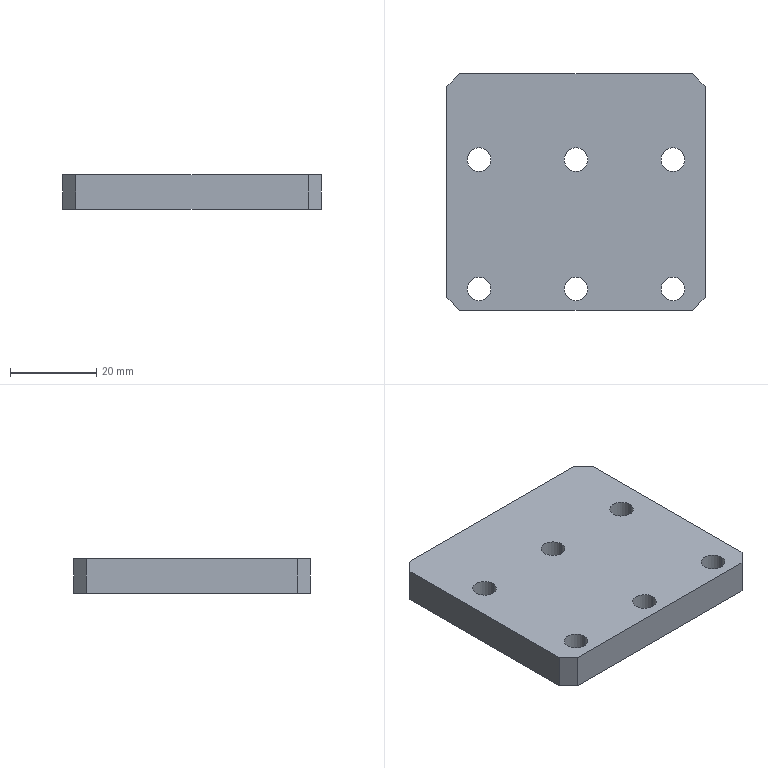Part | SolidWorks | features Chamfer 1, Extrusion 1, HoleWzd 1 | 1 solid | 22 faces | box 60 x 55 x 8 mm | volume 25116 mm3 | cylinder 12 | plane 10 | commonest cylinder face diameters 5.5 x12
STEP:
#1=CARTESIAN_POINT('',(-25.25,-22.5,0.));
#2=VERTEX_POINT('',#1);
#3=CARTESIAN_POINT('',(-19.75,-22.5,0.));
#4=VERTEX_POINT('',#3);
#5=CARTESIAN_POINT('',(-22.5,-22.5,0.));
#6=DIRECTION('',(0.,0.,1.));
#7=DIRECTION('',(1.,0.,0.));
#8=AXIS2_PLACEMENT_3D('',#5,#6,#7);
#9=CIRCLE('',#8,2.75);
#10=EDGE_CURVE('',#2,#4,#9,.T.);
#11=ORIENTED_EDGE('',*,*,#10,.F.);
#12=CARTESIAN_POINT('',(-25.25,-22.5,8.));
#13=VERTEX_POINT('',#12);
#14=CARTESIAN_POINT('',(-25.25,-22.5,8.));
#15=DIRECTION('',(0.,0.,1.));
#16=VECTOR('',#15,1000.);
#17=LINE('',#14,#16);
#18=EDGE_CURVE('',#2,#13,#17,.T.);
#19=ORIENTED_EDGE('',*,*,#18,.T.);
#20=CARTESIAN_POINT('',(-19.75,-22.5,8.));
#21=VERTEX_POINT('',#20);
#22=CARTESIAN_POINT('',(-22.5,-22.5,8.));
#23=DIRECTION('',(0.,0.,1.));
#24=DIRECTION('',(1.,0.,0.));
#25=AXIS2_PLACEMENT_3D('',#22,#23,#24);
#26=CIRCLE('',#25,2.75);
#27=EDGE_CURVE('',#13,#21,#26,.T.);
#28=ORIENTED_EDGE('',*,*,#27,.T.);
#29=CARTESIAN_POINT('',(-19.75,-22.5,8.));
#30=DIRECTION('',(0.,0.,1.));
#31=VECTOR('',#30,1000.);
#32=LINE('',#29,#31);
#33=EDGE_CURVE('',#4,#21,#32,.T.);
#34=ORIENTED_EDGE('',*,*,#33,.F.);
#35=EDGE_LOOP('',(#11,#19,#28,#34));
#36=FACE_OUTER_BOUND('',#35,.T.);
#37=CARTESIAN_POINT('',(-22.5,-22.5,8.));
#38=DIRECTION('',(0.,0.,1.));
#39=DIRECTION('',(1.,0.,0.));
#40=AXIS2_PLACEMENT_3D('',#37,#38,#39);
#41=CYLINDRICAL_SURFACE('',#40,2.75);
#42=ADVANCED_FACE('',(#36),#41,.F.);
#43=CARTESIAN_POINT('',(-25.25,7.5,0.));
#44=VERTEX_POINT('',#43);
#45=CARTESIAN_POINT('',(-19.75,7.5,0.));
#46=VERTEX_POINT('',#45);
#47=CARTESIAN_POINT('',(-22.5,7.5,0.));
#48=DIRECTION('',(0.,0.,1.));
#49=DIRECTION('',(1.,0.,0.));
#50=AXIS2_PLACEMENT_3D('',#47,#48,#49);
#51=CIRCLE('',#50,2.75);
#52=EDGE_CURVE('',#44,#46,#51,.T.);
#53=ORIENTED_EDGE('',*,*,#52,.F.);
#54=CARTESIAN_POINT('',(-25.25,7.5,8.));
#55=VERTEX_POINT('',#54);
#56=CARTESIAN_POINT('',(-25.25,7.5,8.));
#57=DIRECTION('',(0.,0.,1.));
#58=VECTOR('',#57,1000.);
#59=LINE('',#56,#58);
#60=EDGE_CURVE('',#44,#55,#59,.T.);
#61=ORIENTED_EDGE('',*,*,#60,.T.);
#62=CARTESIAN_POINT('',(-19.75,7.5,8.));
#63=VERTEX_POINT('',#62);
#64=CARTESIAN_POINT('',(-22.5,7.5,8.));
#65=DIRECTION('',(0.,0.,1.));
#66=DIRECTION('',(1.,0.,0.));
#67=AXIS2_PLACEMENT_3D('',#64,#65,#66);
#68=CIRCLE('',#67,2.75);
#69=EDGE_CURVE('',#55,#63,#68,.T.);
#70=ORIENTED_EDGE('',*,*,#69,.T.);
#71=CARTESIAN_POINT('',(-19.75,7.5,8.));
#72=DIRECTION('',(0.,0.,1.));
#73=VECTOR('',#72,1000.);
#74=LINE('',#71,#73);
#75=EDGE_CURVE('',#46,#63,#74,.T.);
#76=ORIENTED_EDGE('',*,*,#75,.F.);
#77=EDGE_LOOP('',(#53,#61,#70,#76));
#78=FACE_OUTER_BOUND('',#77,.T.);
#79=CARTESIAN_POINT('',(-22.5,7.5,8.));
#80=DIRECTION('',(0.,0.,1.));
#81=DIRECTION('',(1.,0.,0.));
#82=AXIS2_PLACEMENT_3D('',#79,#80,#81);
#83=CYLINDRICAL_SURFACE('',#82,2.75);
#84=ADVANCED_FACE('',(#78),#83,.F.);
#85=CARTESIAN_POINT('',(-2.75,7.5,0.));
#86=VERTEX_POINT('',#85);
#87=CARTESIAN_POINT('',(2.75,7.5,0.));
#88=VERTEX_POINT('',#87);
#89=CARTESIAN_POINT('',(0.,7.5,0.));
#90=DIRECTION('',(0.,0.,1.));
#91=DIRECTION('',(1.,0.,0.));
#92=AXIS2_PLACEMENT_3D('',#89,#90,#91);
#93=CIRCLE('',#92,2.75);
#94=EDGE_CURVE('',#86,#88,#93,.T.);
#95=ORIENTED_EDGE('',*,*,#94,.F.);
#96=CARTESIAN_POINT('',(-2.75,7.5,8.));
#97=VERTEX_POINT('',#96);
#98=CARTESIAN_POINT('',(-2.75,7.5,8.));
#99=DIRECTION('',(0.,0.,1.));
#100=VECTOR('',#99,1000.);
#101=LINE('',#98,#100);
#102=EDGE_CURVE('',#86,#97,#101,.T.);
#103=ORIENTED_EDGE('',*,*,#102,.T.);
#104=CARTESIAN_POINT('',(2.75,7.5,8.));
#105=VERTEX_POINT('',#104);
#106=CARTESIAN_POINT('',(0.,7.5,8.));
#107=DIRECTION('',(0.,0.,1.));
#108=DIRECTION('',(1.,0.,0.));
#109=AXIS2_PLACEMENT_3D('',#106,#107,#108);
#110=CIRCLE('',#109,2.75);
#111=EDGE_CURVE('',#97,#105,#110,.T.);
#112=ORIENTED_EDGE('',*,*,#111,.T.);
#113=CARTESIAN_POINT('',(2.75,7.5,8.));
#114=DIRECTION('',(0.,0.,1.));
#115=VECTOR('',#114,1000.);
#116=LINE('',#113,#115);
#117=EDGE_CURVE('',#88,#105,#116,.T.);
#118=ORIENTED_EDGE('',*,*,#117,.F.);
#119=EDGE_LOOP('',(#95,#103,#112,#118));
#120=FACE_OUTER_BOUND('',#119,.T.);
#121=CARTESIAN_POINT('',(0.,7.5,8.));
#122=DIRECTION('',(0.,0.,1.));
#123=DIRECTION('',(1.,0.,0.));
#124=AXIS2_PLACEMENT_3D('',#121,#122,#123);
#125=CYLINDRICAL_SURFACE('',#124,2.75);
#126=ADVANCED_FACE('',(#120),#125,.F.);
#127=CARTESIAN_POINT('',(-2.75,-22.5,0.));
#128=VERTEX_POINT('',#127);
#129=CARTESIAN_POINT('',(2.75,-22.5,0.));
#130=VERTEX_POINT('',#129);
#131=CARTESIAN_POINT('',(0.,-22.5,0.));
#132=DIRECTION('',(0.,0.,1.));
#133=DIRECTION('',(1.,0.,0.));
#134=AXIS2_PLACEMENT_3D('',#131,#132,#133);
#135=CIRCLE('',#134,2.75);
#136=EDGE_CURVE('',#128,#130,#135,.T.);
#137=ORIENTED_EDGE('',*,*,#136,.F.);
#138=CARTESIAN_POINT('',(-2.75,-22.5,8.));
#139=VERTEX_POINT('',#138);
#140=CARTESIAN_POINT('',(-2.75,-22.5,8.));
#141=DIRECTION('',(0.,0.,1.));
#142=VECTOR('',#141,1000.);
#143=LINE('',#140,#142);
#144=EDGE_CURVE('',#128,#139,#143,.T.);
#145=ORIENTED_EDGE('',*,*,#144,.T.);
#146=CARTESIAN_POINT('',(2.75,-22.5,8.));
#147=VERTEX_POINT('',#146);
#148=CARTESIAN_POINT('',(0.,-22.5,8.));
#149=DIRECTION('',(0.,0.,1.));
#150=DIRECTION('',(1.,0.,0.));
#151=AXIS2_PLACEMENT_3D('',#148,#149,#150);
#152=CIRCLE('',#151,2.75);
#153=EDGE_CURVE('',#139,#147,#152,.T.);
#154=ORIENTED_EDGE('',*,*,#153,.T.);
#155=CARTESIAN_POINT('',(2.75,-22.5,8.));
#156=DIRECTION('',(0.,0.,1.));
#157=VECTOR('',#156,1000.);
#158=LINE('',#155,#157);
#159=EDGE_CURVE('',#130,#147,#158,.T.);
#160=ORIENTED_EDGE('',*,*,#159,.F.);
#161=EDGE_LOOP('',(#137,#145,#154,#160));
#162=FACE_OUTER_BOUND('',#161,.T.);
#163=CARTESIAN_POINT('',(0.,-22.5,8.));
#164=DIRECTION('',(0.,0.,1.));
#165=DIRECTION('',(1.,0.,0.));
#166=AXIS2_PLACEMENT_3D('',#163,#164,#165);
#167=CYLINDRICAL_SURFACE('',#166,2.75);
#168=ADVANCED_FACE('',(#162),#167,.F.);
#169=CARTESIAN_POINT('',(19.75,-22.5,0.));
#170=VERTEX_POINT('',#169);
#171=CARTESIAN_POINT('',(25.25,-22.5,0.));
#172=VERTEX_POINT('',#171);
#173=CARTESIAN_POINT('',(22.5,-22.5,0.));
#174=DIRECTION('',(0.,0.,1.));
#175=DIRECTION('',(1.,0.,0.));
#176=AXIS2_PLACEMENT_3D('',#173,#174,#175);
#177=CIRCLE('',#176,2.75);
#178=EDGE_CURVE('',#170,#172,#177,.T.);
#179=ORIENTED_EDGE('',*,*,#178,.F.);
#180=CARTESIAN_POINT('',(19.75,-22.5,8.));
#181=VERTEX_POINT('',#180);
#182=CARTESIAN_POINT('',(19.75,-22.5,8.));
#183=DIRECTION('',(0.,0.,1.));
#184=VECTOR('',#183,1000.);
#185=LINE('',#182,#184);
#186=EDGE_CURVE('',#170,#181,#185,.T.);
#187=ORIENTED_EDGE('',*,*,#186,.T.);
#188=CARTESIAN_POINT('',(25.25,-22.5,8.));
#189=VERTEX_POINT('',#188);
#190=CARTESIAN_POINT('',(22.5,-22.5,8.));
#191=DIRECTION('',(0.,0.,1.));
#192=DIRECTION('',(1.,0.,0.));
#193=AXIS2_PLACEMENT_3D('',#190,#191,#192);
#194=CIRCLE('',#193,2.75);
#195=EDGE_CURVE('',#181,#189,#194,.T.);
#196=ORIENTED_EDGE('',*,*,#195,.T.);
#197=CARTESIAN_POINT('',(25.25,-22.5,8.));
#198=DIRECTION('',(0.,0.,1.));
#199=VECTOR('',#198,1000.);
#200=LINE('',#197,#199);
#201=EDGE_CURVE('',#172,#189,#200,.T.);
#202=ORIENTED_EDGE('',*,*,#201,.F.);
#203=EDGE_LOOP('',(#179,#187,#196,#202));
#204=FACE_OUTER_BOUND('',#203,.T.);
#205=CARTESIAN_POINT('',(22.5,-22.5,8.));
#206=DIRECTION('',(0.,0.,1.));
#207=DIRECTION('',(1.,0.,0.));
#208=AXIS2_PLACEMENT_3D('',#205,#206,#207);
#209=CYLINDRICAL_SURFACE('',#208,2.75);
#210=ADVANCED_FACE('',(#204),#209,.F.);
#211=CARTESIAN_POINT('',(19.75,7.5,0.));
#212=VERTEX_POINT('',#211);
#213=CARTESIAN_POINT('',(25.25,7.5,0.));
#214=VERTEX_POINT('',#213);
#215=CARTESIAN_POINT('',(22.5,7.5,0.));
#216=DIRECTION('',(0.,0.,1.));
#217=DIRECTION('',(1.,0.,0.));
#218=AXIS2_PLACEMENT_3D('',#215,#216,#217);
#219=CIRCLE('',#218,2.75);
#220=EDGE_CURVE('',#212,#214,#219,.T.);
#221=ORIENTED_EDGE('',*,*,#220,.F.);
#222=CARTESIAN_POINT('',(19.75,7.5,8.));
#223=VERTEX_POINT('',#222);
#224=CARTESIAN_POINT('',(19.75,7.5,8.));
#225=DIRECTION('',(0.,0.,1.));
#226=VECTOR('',#225,1000.);
#227=LINE('',#224,#226);
#228=EDGE_CURVE('',#212,#223,#227,.T.);
#229=ORIENTED_EDGE('',*,*,#228,.T.);
#230=CARTESIAN_POINT('',(25.25,7.5,8.));
#231=VERTEX_POINT('',#230);
#232=CARTESIAN_POINT('',(22.5,7.5,8.));
#233=DIRECTION('',(0.,0.,1.));
#234=DIRECTION('',(1.,0.,0.));
#235=AXIS2_PLACEMENT_3D('',#232,#233,#234);
#236=CIRCLE('',#235,2.75);
#237=EDGE_CURVE('',#223,#231,#236,.T.);
#238=ORIENTED_EDGE('',*,*,#237,.T.);
#239=CARTESIAN_POINT('',(25.25,7.5,8.));
#240=DIRECTION('',(0.,0.,1.));
#241=VECTOR('',#240,1000.);
#242=LINE('',#239,#241);
#243=EDGE_CURVE('',#214,#231,#242,.T.);
#244=ORIENTED_EDGE('',*,*,#243,.F.);
#245=EDGE_LOOP('',(#221,#229,#238,#244));
#246=FACE_OUTER_BOUND('',#245,.T.);
#247=CARTESIAN_POINT('',(22.5,7.5,8.));
#248=DIRECTION('',(0.,0.,1.));
#249=DIRECTION('',(1.,0.,0.));
#250=AXIS2_PLACEMENT_3D('',#247,#248,#249);
#251=CYLINDRICAL_SURFACE('',#250,2.75);
#252=ADVANCED_FACE('',(#246),#251,.F.);
#253=CARTESIAN_POINT('',(30.,-24.5,0.));
#254=VERTEX_POINT('',#253);
#255=CARTESIAN_POINT('',(30.,24.5,0.));
#256=VERTEX_POINT('',#255);
#257=CARTESIAN_POINT('',(30.,27.5,0.));
#258=DIRECTION('',(0.,1.,0.));
#259=VECTOR('',#258,1000.);
#260=LINE('',#257,#259);
#261=EDGE_CURVE('',#254,#256,#260,.T.);
#262=ORIENTED_EDGE('',*,*,#261,.T.);
#263=CARTESIAN_POINT('',(30.,24.5,8.));
#264=VERTEX_POINT('',#263);
#265=CARTESIAN_POINT('',(30.,24.5,8.));
#266=DIRECTION('',(0.,0.,1.));
#267=VECTOR('',#266,1000.);
#268=LINE('',#265,#267);
#269=EDGE_CURVE('',#256,#264,#268,.T.);
#270=ORIENTED_EDGE('',*,*,#269,.T.);
#271=CARTESIAN_POINT('',(30.,-24.5,8.));
#272=VERTEX_POINT('',#271);
#273=CARTESIAN_POINT('',(30.,27.5,8.));
#274=DIRECTION('',(0.,1.,0.));
#275=VECTOR('',#274,1000.);
#276=LINE('',#273,#275);
#277=EDGE_CURVE('',#272,#264,#276,.T.);
#278=ORIENTED_EDGE('',*,*,#277,.F.);
#279=CARTESIAN_POINT('',(30.,-24.5,8.));
#280=DIRECTION('',(0.,0.,-1.));
#281=VECTOR('',#280,1000.);
#282=LINE('',#279,#281);
#283=EDGE_CURVE('',#272,#254,#282,.T.);
#284=ORIENTED_EDGE('',*,*,#283,.T.);
#285=EDGE_LOOP('',(#262,#270,#278,#284));
#286=FACE_OUTER_BOUND('',#285,.T.);
#287=CARTESIAN_POINT('',(30.,27.5,8.));
#288=DIRECTION('',(-1.,0.,0.));
#289=DIRECTION('',(0.,-1.,0.));
#290=AXIS2_PLACEMENT_3D('',#287,#288,#289);
#291=PLANE('',#290);
#292=ADVANCED_FACE('',(#286),#291,.F.);
#293=CARTESIAN_POINT('',(27.,27.5,8.));
#294=VERTEX_POINT('',#293);
#295=CARTESIAN_POINT('',(-27.,27.5,8.));
#296=VERTEX_POINT('',#295);
#297=CARTESIAN_POINT('',(-30.,27.5,8.));
#298=DIRECTION('',(-1.,0.,0.));
#299=VECTOR('',#298,1000.);
#300=LINE('',#297,#299);
#301=EDGE_CURVE('',#294,#296,#300,.T.);
#302=ORIENTED_EDGE('',*,*,#301,.F.);
#303=CARTESIAN_POINT('',(27.,27.5,0.));
#304=VERTEX_POINT('',#303);
#305=CARTESIAN_POINT('',(27.,27.5,8.));
#306=DIRECTION('',(0.,0.,-1.));
#307=VECTOR('',#306,1000.);
#308=LINE('',#305,#307);
#309=EDGE_CURVE('',#294,#304,#308,.T.);
#310=ORIENTED_EDGE('',*,*,#309,.T.);
#311=CARTESIAN_POINT('',(-27.,27.5,0.));
#312=VERTEX_POINT('',#311);
#313=CARTESIAN_POINT('',(-30.,27.5,0.));
#314=DIRECTION('',(-1.,0.,0.));
#315=VECTOR('',#314,1000.);
#316=LINE('',#313,#315);
#317=EDGE_CURVE('',#304,#312,#316,.T.);
#318=ORIENTED_EDGE('',*,*,#317,.T.);
#319=CARTESIAN_POINT('',(-27.,27.5,8.));
#320=DIRECTION('',(0.,0.,1.));
#321=VECTOR('',#320,1000.);
#322=LINE('',#319,#321);
#323=EDGE_CURVE('',#312,#296,#322,.T.);
#324=ORIENTED_EDGE('',*,*,#323,.T.);
#325=EDGE_LOOP('',(#302,#310,#318,#324));
#326=FACE_OUTER_BOUND('',#325,.T.);
#327=CARTESIAN_POINT('',(-30.,27.5,8.));
#328=DIRECTION('',(0.,-1.,0.));
#329=DIRECTION('',(0.,0.,-1.));
#330=AXIS2_PLACEMENT_3D('',#327,#328,#329);
#331=PLANE('',#330);
#332=ADVANCED_FACE('',(#326),#331,.F.);
#333=CARTESIAN_POINT('',(-30.,24.5,8.));
#334=VERTEX_POINT('',#333);
#335=CARTESIAN_POINT('',(-30.,-24.5,8.));
#336=VERTEX_POINT('',#335);
#337=CARTESIAN_POINT('',(-30.,27.5,8.));
#338=DIRECTION('',(0.,-1.,0.));
#339=VECTOR('',#338,1000.);
#340=LINE('',#337,#339);
#341=EDGE_CURVE('',#334,#336,#340,.T.);
#342=ORIENTED_EDGE('',*,*,#341,.F.);
#343=CARTESIAN_POINT('',(-30.,24.5,0.));
#344=VERTEX_POINT('',#343);
#345=CARTESIAN_POINT('',(-30.,24.5,8.));
#346=DIRECTION('',(0.,0.,-1.));
#347=VECTOR('',#346,1000.);
#348=LINE('',#345,#347);
#349=EDGE_CURVE('',#334,#344,#348,.T.);
#350=ORIENTED_EDGE('',*,*,#349,.T.);
#351=CARTESIAN_POINT('',(-30.,-24.5,0.));
#352=VERTEX_POINT('',#351);
#353=CARTESIAN_POINT('',(-30.,27.5,0.));
#354=DIRECTION('',(0.,-1.,0.));
#355=VECTOR('',#354,1000.);
#356=LINE('',#353,#355);
#357=EDGE_CURVE('',#344,#352,#356,.T.);
#358=ORIENTED_EDGE('',*,*,#357,.T.);
#359=CARTESIAN_POINT('',(-30.,-24.5,8.));
#360=DIRECTION('',(0.,0.,1.));
#361=VECTOR('',#360,1000.);
#362=LINE('',#359,#361);
#363=EDGE_CURVE('',#352,#336,#362,.T.);
#364=ORIENTED_EDGE('',*,*,#363,.T.);
#365=EDGE_LOOP('',(#342,#350,#358,#364));
#366=FACE_OUTER_BOUND('',#365,.T.);
#367=CARTESIAN_POINT('',(-30.,27.5,8.));
#368=DIRECTION('',(1.,0.,0.));
#369=DIRECTION('',(0.,1.,0.));
#370=AXIS2_PLACEMENT_3D('',#367,#368,#369);
#371=PLANE('',#370);
#372=ADVANCED_FACE('',(#366),#371,.F.);
#373=CARTESIAN_POINT('',(-27.,-27.5,8.));
#374=VERTEX_POINT('',#373);
#375=CARTESIAN_POINT('',(27.,-27.5,8.));
#376=VERTEX_POINT('',#375);
#377=CARTESIAN_POINT('',(-30.,-27.5,8.));
#378=DIRECTION('',(1.,0.,0.));
#379=VECTOR('',#378,1000.);
#380=LINE('',#377,#379);
#381=EDGE_CURVE('',#374,#376,#380,.T.);
#382=ORIENTED_EDGE('',*,*,#381,.F.);
#383=CARTESIAN_POINT('',(-27.,-27.5,0.));
#384=VERTEX_POINT('',#383);
#385=CARTESIAN_POINT('',(-27.,-27.5,8.));
#386=DIRECTION('',(0.,0.,-1.));
#387=VECTOR('',#386,1000.);
#388=LINE('',#385,#387);
#389=EDGE_CURVE('',#374,#384,#388,.T.);
#390=ORIENTED_EDGE('',*,*,#389,.T.);
#391=CARTESIAN_POINT('',(27.,-27.5,0.));
#392=VERTEX_POINT('',#391);
#393=CARTESIAN_POINT('',(-30.,-27.5,0.));
#394=DIRECTION('',(1.,0.,0.));
#395=VECTOR('',#394,1000.);
#396=LINE('',#393,#395);
#397=EDGE_CURVE('',#384,#392,#396,.T.);
#398=ORIENTED_EDGE('',*,*,#397,.T.);
#399=CARTESIAN_POINT('',(27.,-27.5,8.));
#400=DIRECTION('',(0.,0.,1.));
#401=VECTOR('',#400,1000.);
#402=LINE('',#399,#401);
#403=EDGE_CURVE('',#392,#376,#402,.T.);
#404=ORIENTED_EDGE('',*,*,#403,.T.);
#405=EDGE_LOOP('',(#382,#390,#398,#404));
#406=FACE_OUTER_BOUND('',#405,.T.);
#407=CARTESIAN_POINT('',(-30.,-27.5,8.));
#408=DIRECTION('',(0.,1.,0.));
#409=DIRECTION('',(0.,0.,1.));
#410=AXIS2_PLACEMENT_3D('',#407,#408,#409);
#411=PLANE('',#410);
#412=ADVANCED_FACE('',(#406),#411,.F.);
#413=CARTESIAN_POINT('',(-22.5,-22.5,8.));
#414=DIRECTION('',(0.,0.,1.));
#415=DIRECTION('',(1.,0.,0.));
#416=AXIS2_PLACEMENT_3D('',#413,#414,#415);
#417=CIRCLE('',#416,2.75);
#418=EDGE_CURVE('',#21,#13,#417,.T.);
#419=ORIENTED_EDGE('',*,*,#418,.F.);
#420=ORIENTED_EDGE('',*,*,#27,.F.);
#421=EDGE_LOOP('',(#419,#420));
#422=FACE_BOUND('',#421,.T.);
#423=CARTESIAN_POINT('',(-22.5,7.5,8.));
#424=DIRECTION('',(0.,0.,1.));
#425=DIRECTION('',(1.,0.,0.));
#426=AXIS2_PLACEMENT_3D('',#423,#424,#425);
#427=CIRCLE('',#426,2.75);
#428=EDGE_CURVE('',#63,#55,#427,.T.);
#429=ORIENTED_EDGE('',*,*,#428,.F.);
#430=ORIENTED_EDGE('',*,*,#69,.F.);
#431=EDGE_LOOP('',(#429,#430));
#432=FACE_BOUND('',#431,.T.);
#433=CARTESIAN_POINT('',(0.,7.5,8.));
#434=DIRECTION('',(0.,0.,1.));
#435=DIRECTION('',(1.,0.,0.));
#436=AXIS2_PLACEMENT_3D('',#433,#434,#435);
#437=CIRCLE('',#436,2.75);
#438=EDGE_CURVE('',#105,#97,#437,.T.);
#439=ORIENTED_EDGE('',*,*,#438,.F.);
#440=ORIENTED_EDGE('',*,*,#111,.F.);
#441=EDGE_LOOP('',(#439,#440));
#442=FACE_BOUND('',#441,.T.);
#443=CARTESIAN_POINT('',(0.,-22.5,8.));
#444=DIRECTION('',(0.,0.,1.));
#445=DIRECTION('',(1.,0.,0.));
#446=AXIS2_PLACEMENT_3D('',#443,#444,#445);
#447=CIRCLE('',#446,2.75);
#448=EDGE_CURVE('',#147,#139,#447,.T.);
#449=ORIENTED_EDGE('',*,*,#448,.F.);
#450=ORIENTED_EDGE('',*,*,#153,.F.);
#451=EDGE_LOOP('',(#449,#450));
#452=FACE_BOUND('',#451,.T.);
#453=CARTESIAN_POINT('',(22.5,-22.5,8.));
#454=DIRECTION('',(0.,0.,1.));
#455=DIRECTION('',(1.,0.,0.));
#456=AXIS2_PLACEMENT_3D('',#453,#454,#455);
#457=CIRCLE('',#456,2.75);
#458=EDGE_CURVE('',#189,#181,#457,.T.);
#459=ORIENTED_EDGE('',*,*,#458,.F.);
#460=ORIENTED_EDGE('',*,*,#195,.F.);
#461=EDGE_LOOP('',(#459,#460));
#462=FACE_BOUND('',#461,.T.);
#463=CARTESIAN_POINT('',(22.5,7.5,8.));
#464=DIRECTION('',(0.,0.,1.));
#465=DIRECTION('',(1.,0.,0.));
#466=AXIS2_PLACEMENT_3D('',#463,#464,#465);
#467=CIRCLE('',#466,2.75);
#468=EDGE_CURVE('',#231,#223,#467,.T.);
#469=ORIENTED_EDGE('',*,*,#468,.F.);
#470=ORIENTED_EDGE('',*,*,#237,.F.);
#471=EDGE_LOOP('',(#469,#470));
#472=FACE_BOUND('',#471,.T.);
#473=ORIENTED_EDGE('',*,*,#277,.T.);
#474=CARTESIAN_POINT('',(27.25,27.25,8.));
#475=DIRECTION('',(-0.7071,0.7071,0.));
#476=VECTOR('',#475,1000.);
#477=LINE('',#474,#476);
#478=EDGE_CURVE('',#264,#294,#477,.T.);
#479=ORIENTED_EDGE('',*,*,#478,.T.);
#480=ORIENTED_EDGE('',*,*,#301,.T.);
#481=CARTESIAN_POINT('',(-27.25,27.25,8.));
#482=DIRECTION('',(-0.7071,-0.7071,0.));
#483=VECTOR('',#482,1000.);
#484=LINE('',#481,#483);
#485=EDGE_CURVE('',#296,#334,#484,.T.);
#486=ORIENTED_EDGE('',*,*,#485,.T.);
#487=ORIENTED_EDGE('',*,*,#341,.T.);
#488=CARTESIAN_POINT('',(-27.25,-27.25,8.));
#489=DIRECTION('',(0.7071,-0.7071,0.));
#490=VECTOR('',#489,1000.);
#491=LINE('',#488,#490);
#492=EDGE_CURVE('',#336,#374,#491,.T.);
#493=ORIENTED_EDGE('',*,*,#492,.T.);
#494=ORIENTED_EDGE('',*,*,#381,.T.);
#495=CARTESIAN_POINT('',(27.25,-27.25,8.));
#496=DIRECTION('',(0.7071,0.7071,0.));
#497=VECTOR('',#496,1000.);
#498=LINE('',#495,#497);
#499=EDGE_CURVE('',#376,#272,#498,.T.);
#500=ORIENTED_EDGE('',*,*,#499,.T.);
#501=EDGE_LOOP('',(#473,#479,#480,#486,#487,#493,#494,#500));
#502=FACE_OUTER_BOUND('',#501,.T.);
#503=CARTESIAN_POINT('',(0.,0.,8.));
#504=DIRECTION('',(0.,0.,1.));
#505=DIRECTION('',(1.,0.,0.));
#506=AXIS2_PLACEMENT_3D('',#503,#504,#505);
#507=PLANE('',#506);
#508=ADVANCED_FACE('',(#422,#432,#442,#452,#462,#472,#502),#507,.T.);
#509=CARTESIAN_POINT('',(-22.5,-22.5,0.));
#510=DIRECTION('',(0.,0.,1.));
#511=DIRECTION('',(1.,0.,0.));
#512=AXIS2_PLACEMENT_3D('',#509,#510,#511);
#513=CIRCLE('',#512,2.75);
#514=EDGE_CURVE('',#4,#2,#513,.T.);
#515=ORIENTED_EDGE('',*,*,#514,.T.);
#516=ORIENTED_EDGE('',*,*,#10,.T.);
#517=EDGE_LOOP('',(#515,#516));
#518=FACE_BOUND('',#517,.T.);
#519=CARTESIAN_POINT('',(-22.5,7.5,0.));
#520=DIRECTION('',(0.,0.,1.));
#521=DIRECTION('',(1.,0.,0.));
#522=AXIS2_PLACEMENT_3D('',#519,#520,#521);
#523=CIRCLE('',#522,2.75);
#524=EDGE_CURVE('',#46,#44,#523,.T.);
#525=ORIENTED_EDGE('',*,*,#524,.T.);
#526=ORIENTED_EDGE('',*,*,#52,.T.);
#527=EDGE_LOOP('',(#525,#526));
#528=FACE_BOUND('',#527,.T.);
#529=CARTESIAN_POINT('',(0.,7.5,0.));
#530=DIRECTION('',(0.,0.,1.));
#531=DIRECTION('',(1.,0.,0.));
#532=AXIS2_PLACEMENT_3D('',#529,#530,#531);
#533=CIRCLE('',#532,2.75);
#534=EDGE_CURVE('',#88,#86,#533,.T.);
#535=ORIENTED_EDGE('',*,*,#534,.T.);
#536=ORIENTED_EDGE('',*,*,#94,.T.);
#537=EDGE_LOOP('',(#535,#536));
#538=FACE_BOUND('',#537,.T.);
#539=CARTESIAN_POINT('',(0.,-22.5,0.));
#540=DIRECTION('',(0.,0.,1.));
#541=DIRECTION('',(1.,0.,0.));
#542=AXIS2_PLACEMENT_3D('',#539,#540,#541);
#543=CIRCLE('',#542,2.75);
#544=EDGE_CURVE('',#130,#128,#543,.T.);
#545=ORIENTED_EDGE('',*,*,#544,.T.);
#546=ORIENTED_EDGE('',*,*,#136,.T.);
#547=EDGE_LOOP('',(#545,#546));
#548=FACE_BOUND('',#547,.T.);
#549=CARTESIAN_POINT('',(22.5,-22.5,0.));
#550=DIRECTION('',(0.,0.,1.));
#551=DIRECTION('',(1.,0.,0.));
#552=AXIS2_PLACEMENT_3D('',#549,#550,#551);
#553=CIRCLE('',#552,2.75);
#554=EDGE_CURVE('',#172,#170,#553,.T.);
#555=ORIENTED_EDGE('',*,*,#554,.T.);
#556=ORIENTED_EDGE('',*,*,#178,.T.);
#557=EDGE_LOOP('',(#555,#556));
#558=FACE_BOUND('',#557,.T.);
#559=CARTESIAN_POINT('',(22.5,7.5,0.));
#560=DIRECTION('',(0.,0.,1.));
#561=DIRECTION('',(1.,0.,0.));
#562=AXIS2_PLACEMENT_3D('',#559,#560,#561);
#563=CIRCLE('',#562,2.75);
#564=EDGE_CURVE('',#214,#212,#563,.T.);
#565=ORIENTED_EDGE('',*,*,#564,.T.);
#566=ORIENTED_EDGE('',*,*,#220,.T.);
#567=EDGE_LOOP('',(#565,#566));
#568=FACE_BOUND('',#567,.T.);
#569=ORIENTED_EDGE('',*,*,#317,.F.);
#570=CARTESIAN_POINT('',(27.,27.5,0.));
#571=DIRECTION('',(0.7071,-0.7071,0.));
#572=VECTOR('',#571,1000.);
#573=LINE('',#570,#572);
#574=EDGE_CURVE('',#304,#256,#573,.T.);
#575=ORIENTED_EDGE('',*,*,#574,.T.);
#576=ORIENTED_EDGE('',*,*,#261,.F.);
#577=CARTESIAN_POINT('',(30.,-24.5,0.));
#578=DIRECTION('',(-0.7071,-0.7071,0.));
#579=VECTOR('',#578,1000.);
#580=LINE('',#577,#579);
#581=EDGE_CURVE('',#254,#392,#580,.T.);
#582=ORIENTED_EDGE('',*,*,#581,.T.);
#583=ORIENTED_EDGE('',*,*,#397,.F.);
#584=CARTESIAN_POINT('',(-27.,-27.5,0.));
#585=DIRECTION('',(-0.7071,0.7071,0.));
#586=VECTOR('',#585,1000.);
#587=LINE('',#584,#586);
#588=EDGE_CURVE('',#384,#352,#587,.T.);
#589=ORIENTED_EDGE('',*,*,#588,.T.);
#590=ORIENTED_EDGE('',*,*,#357,.F.);
#591=CARTESIAN_POINT('',(-30.,24.5,0.));
#592=DIRECTION('',(0.7071,0.7071,0.));
#593=VECTOR('',#592,1000.);
#594=LINE('',#591,#593);
#595=EDGE_CURVE('',#344,#312,#594,.T.);
#596=ORIENTED_EDGE('',*,*,#595,.T.);
#597=EDGE_LOOP('',(#569,#575,#576,#582,#583,#589,#590,#596));
#598=FACE_OUTER_BOUND('',#597,.T.);
#599=CARTESIAN_POINT('',(0.,0.,0.));
#600=DIRECTION('',(0.,0.,1.));
#601=DIRECTION('',(1.,0.,0.));
#602=AXIS2_PLACEMENT_3D('',#599,#600,#601);
#603=PLANE('',#602);
#604=ADVANCED_FACE('',(#518,#528,#538,#548,#558,#568,#598),#603,.F.);
#605=ORIENTED_EDGE('',*,*,#228,.F.);
#606=ORIENTED_EDGE('',*,*,#564,.F.);
#607=ORIENTED_EDGE('',*,*,#243,.T.);
#608=ORIENTED_EDGE('',*,*,#468,.T.);
#609=EDGE_LOOP('',(#605,#606,#607,#608));
#610=FACE_OUTER_BOUND('',#609,.T.);
#611=CARTESIAN_POINT('',(22.5,7.5,8.));
#612=DIRECTION('',(0.,0.,1.));
#613=DIRECTION('',(1.,0.,0.));
#614=AXIS2_PLACEMENT_3D('',#611,#612,#613);
#615=CYLINDRICAL_SURFACE('',#614,2.75);
#616=ADVANCED_FACE('',(#610),#615,.F.);
#617=ORIENTED_EDGE('',*,*,#186,.F.);
#618=ORIENTED_EDGE('',*,*,#554,.F.);
#619=ORIENTED_EDGE('',*,*,#201,.T.);
#620=ORIENTED_EDGE('',*,*,#458,.T.);
#621=EDGE_LOOP('',(#617,#618,#619,#620));
#622=FACE_OUTER_BOUND('',#621,.T.);
#623=CARTESIAN_POINT('',(22.5,-22.5,8.));
#624=DIRECTION('',(0.,0.,1.));
#625=DIRECTION('',(1.,0.,0.));
#626=AXIS2_PLACEMENT_3D('',#623,#624,#625);
#627=CYLINDRICAL_SURFACE('',#626,2.75);
#628=ADVANCED_FACE('',(#622),#627,.F.);
#629=ORIENTED_EDGE('',*,*,#144,.F.);
#630=ORIENTED_EDGE('',*,*,#544,.F.);
#631=ORIENTED_EDGE('',*,*,#159,.T.);
#632=ORIENTED_EDGE('',*,*,#448,.T.);
#633=EDGE_LOOP('',(#629,#630,#631,#632));
#634=FACE_OUTER_BOUND('',#633,.T.);
#635=CARTESIAN_POINT('',(0.,-22.5,8.));
#636=DIRECTION('',(0.,0.,1.));
#637=DIRECTION('',(1.,0.,0.));
#638=AXIS2_PLACEMENT_3D('',#635,#636,#637);
#639=CYLINDRICAL_SURFACE('',#638,2.75);
#640=ADVANCED_FACE('',(#634),#639,.F.);
#641=ORIENTED_EDGE('',*,*,#102,.F.);
#642=ORIENTED_EDGE('',*,*,#534,.F.);
#643=ORIENTED_EDGE('',*,*,#117,.T.);
#644=ORIENTED_EDGE('',*,*,#438,.T.);
#645=EDGE_LOOP('',(#641,#642,#643,#644));
#646=FACE_OUTER_BOUND('',#645,.T.);
#647=CARTESIAN_POINT('',(0.,7.5,8.));
#648=DIRECTION('',(0.,0.,1.));
#649=DIRECTION('',(1.,0.,0.));
#650=AXIS2_PLACEMENT_3D('',#647,#648,#649);
#651=CYLINDRICAL_SURFACE('',#650,2.75);
#652=ADVANCED_FACE('',(#646),#651,.F.);
#653=ORIENTED_EDGE('',*,*,#60,.F.);
#654=ORIENTED_EDGE('',*,*,#524,.F.);
#655=ORIENTED_EDGE('',*,*,#75,.T.);
#656=ORIENTED_EDGE('',*,*,#428,.T.);
#657=EDGE_LOOP('',(#653,#654,#655,#656));
#658=FACE_OUTER_BOUND('',#657,.T.);
#659=CARTESIAN_POINT('',(-22.5,7.5,8.));
#660=DIRECTION('',(0.,0.,1.));
#661=DIRECTION('',(1.,0.,0.));
#662=AXIS2_PLACEMENT_3D('',#659,#660,#661);
#663=CYLINDRICAL_SURFACE('',#662,2.75);
#664=ADVANCED_FACE('',(#658),#663,.F.);
#665=ORIENTED_EDGE('',*,*,#18,.F.);
#666=ORIENTED_EDGE('',*,*,#514,.F.);
#667=ORIENTED_EDGE('',*,*,#33,.T.);
#668=ORIENTED_EDGE('',*,*,#418,.T.);
#669=EDGE_LOOP('',(#665,#666,#667,#668));
#670=FACE_OUTER_BOUND('',#669,.T.);
#671=CARTESIAN_POINT('',(-22.5,-22.5,8.));
#672=DIRECTION('',(0.,0.,1.));
#673=DIRECTION('',(1.,0.,0.));
#674=AXIS2_PLACEMENT_3D('',#671,#672,#673);
#675=CYLINDRICAL_SURFACE('',#674,2.75);
#676=ADVANCED_FACE('',(#670),#675,.F.);
#677=ORIENTED_EDGE('',*,*,#478,.F.);
#678=ORIENTED_EDGE('',*,*,#269,.F.);
#679=ORIENTED_EDGE('',*,*,#574,.F.);
#680=ORIENTED_EDGE('',*,*,#309,.F.);
#681=EDGE_LOOP('',(#677,#678,#679,#680));
#682=FACE_OUTER_BOUND('',#681,.T.);
#683=CARTESIAN_POINT('',(27.,27.5,8.));
#684=DIRECTION('',(-0.7071,-0.7071,0.));
#685=DIRECTION('',(0.,0.,-1.));
#686=AXIS2_PLACEMENT_3D('',#683,#684,#685);
#687=PLANE('',#686);
#688=ADVANCED_FACE('',(#682),#687,.F.);
#689=ORIENTED_EDGE('',*,*,#485,.F.);
#690=ORIENTED_EDGE('',*,*,#323,.F.);
#691=ORIENTED_EDGE('',*,*,#595,.F.);
#692=ORIENTED_EDGE('',*,*,#349,.F.);
#693=EDGE_LOOP('',(#689,#690,#691,#692));
#694=FACE_OUTER_BOUND('',#693,.T.);
#695=CARTESIAN_POINT('',(-30.,24.5,8.));
#696=DIRECTION('',(0.7071,-0.7071,0.));
#697=DIRECTION('',(0.,0.,-1.));
#698=AXIS2_PLACEMENT_3D('',#695,#696,#697);
#699=PLANE('',#698);
#700=ADVANCED_FACE('',(#694),#699,.F.);
#701=ORIENTED_EDGE('',*,*,#492,.F.);
#702=ORIENTED_EDGE('',*,*,#363,.F.);
#703=ORIENTED_EDGE('',*,*,#588,.F.);
#704=ORIENTED_EDGE('',*,*,#389,.F.);
#705=EDGE_LOOP('',(#701,#702,#703,#704));
#706=FACE_OUTER_BOUND('',#705,.T.);
#707=CARTESIAN_POINT('',(-27.,-27.5,8.));
#708=DIRECTION('',(0.7071,0.7071,0.));
#709=DIRECTION('',(0.,0.,-1.));
#710=AXIS2_PLACEMENT_3D('',#707,#708,#709);
#711=PLANE('',#710);
#712=ADVANCED_FACE('',(#706),#711,.F.);
#713=ORIENTED_EDGE('',*,*,#499,.F.);
#714=ORIENTED_EDGE('',*,*,#403,.F.);
#715=ORIENTED_EDGE('',*,*,#581,.F.);
#716=ORIENTED_EDGE('',*,*,#283,.F.);
#717=EDGE_LOOP('',(#713,#714,#715,#716));
#718=FACE_OUTER_BOUND('',#717,.T.);
#719=CARTESIAN_POINT('',(30.,-24.5,8.));
#720=DIRECTION('',(-0.7071,0.7071,0.));
#721=DIRECTION('',(0.,0.,-1.));
#722=AXIS2_PLACEMENT_3D('',#719,#720,#721);
#723=PLANE('',#722);
#724=ADVANCED_FACE('',(#718),#723,.F.);
#725=CLOSED_SHELL('',(#42,#84,#126,#168,#210,#252,#292,#332,#372,#412,#508,#604,#616,#628,#640,#652,#664,#676,#688,#700,#712,#724));
#726=MANIFOLD_SOLID_BREP('',#725);
#727=CARTESIAN_POINT('',(0.,0.,0.));
#728=DIRECTION('',(0.,0.,1.));
#729=DIRECTION('',(1.,0.,0.));
#730=AXIS2_PLACEMENT_3D('',#727,#728,#729);
#731=(LENGTH_UNIT()NAMED_UNIT(*)SI_UNIT(.MILLI.,.METRE.));
#732=UNCERTAINTY_MEASURE_WITH_UNIT(LENGTH_MEASURE(0.00001),#731,'','');
#733=(NAMED_UNIT(*)PLANE_ANGLE_UNIT()SI_UNIT($,.RADIAN.));
#734=(NAMED_UNIT(*)SI_UNIT($,.STERADIAN.)SOLID_ANGLE_UNIT());
#735=(GEOMETRIC_REPRESENTATION_CONTEXT(3)GLOBAL_UNCERTAINTY_ASSIGNED_CONTEXT((#732))GLOBAL_UNIT_ASSIGNED_CONTEXT((#731,#733,#734))REPRESENTATION_CONTEXT('',''));
#736=ADVANCED_BREP_SHAPE_REPRESENTATION('',(#726,#730),#735);